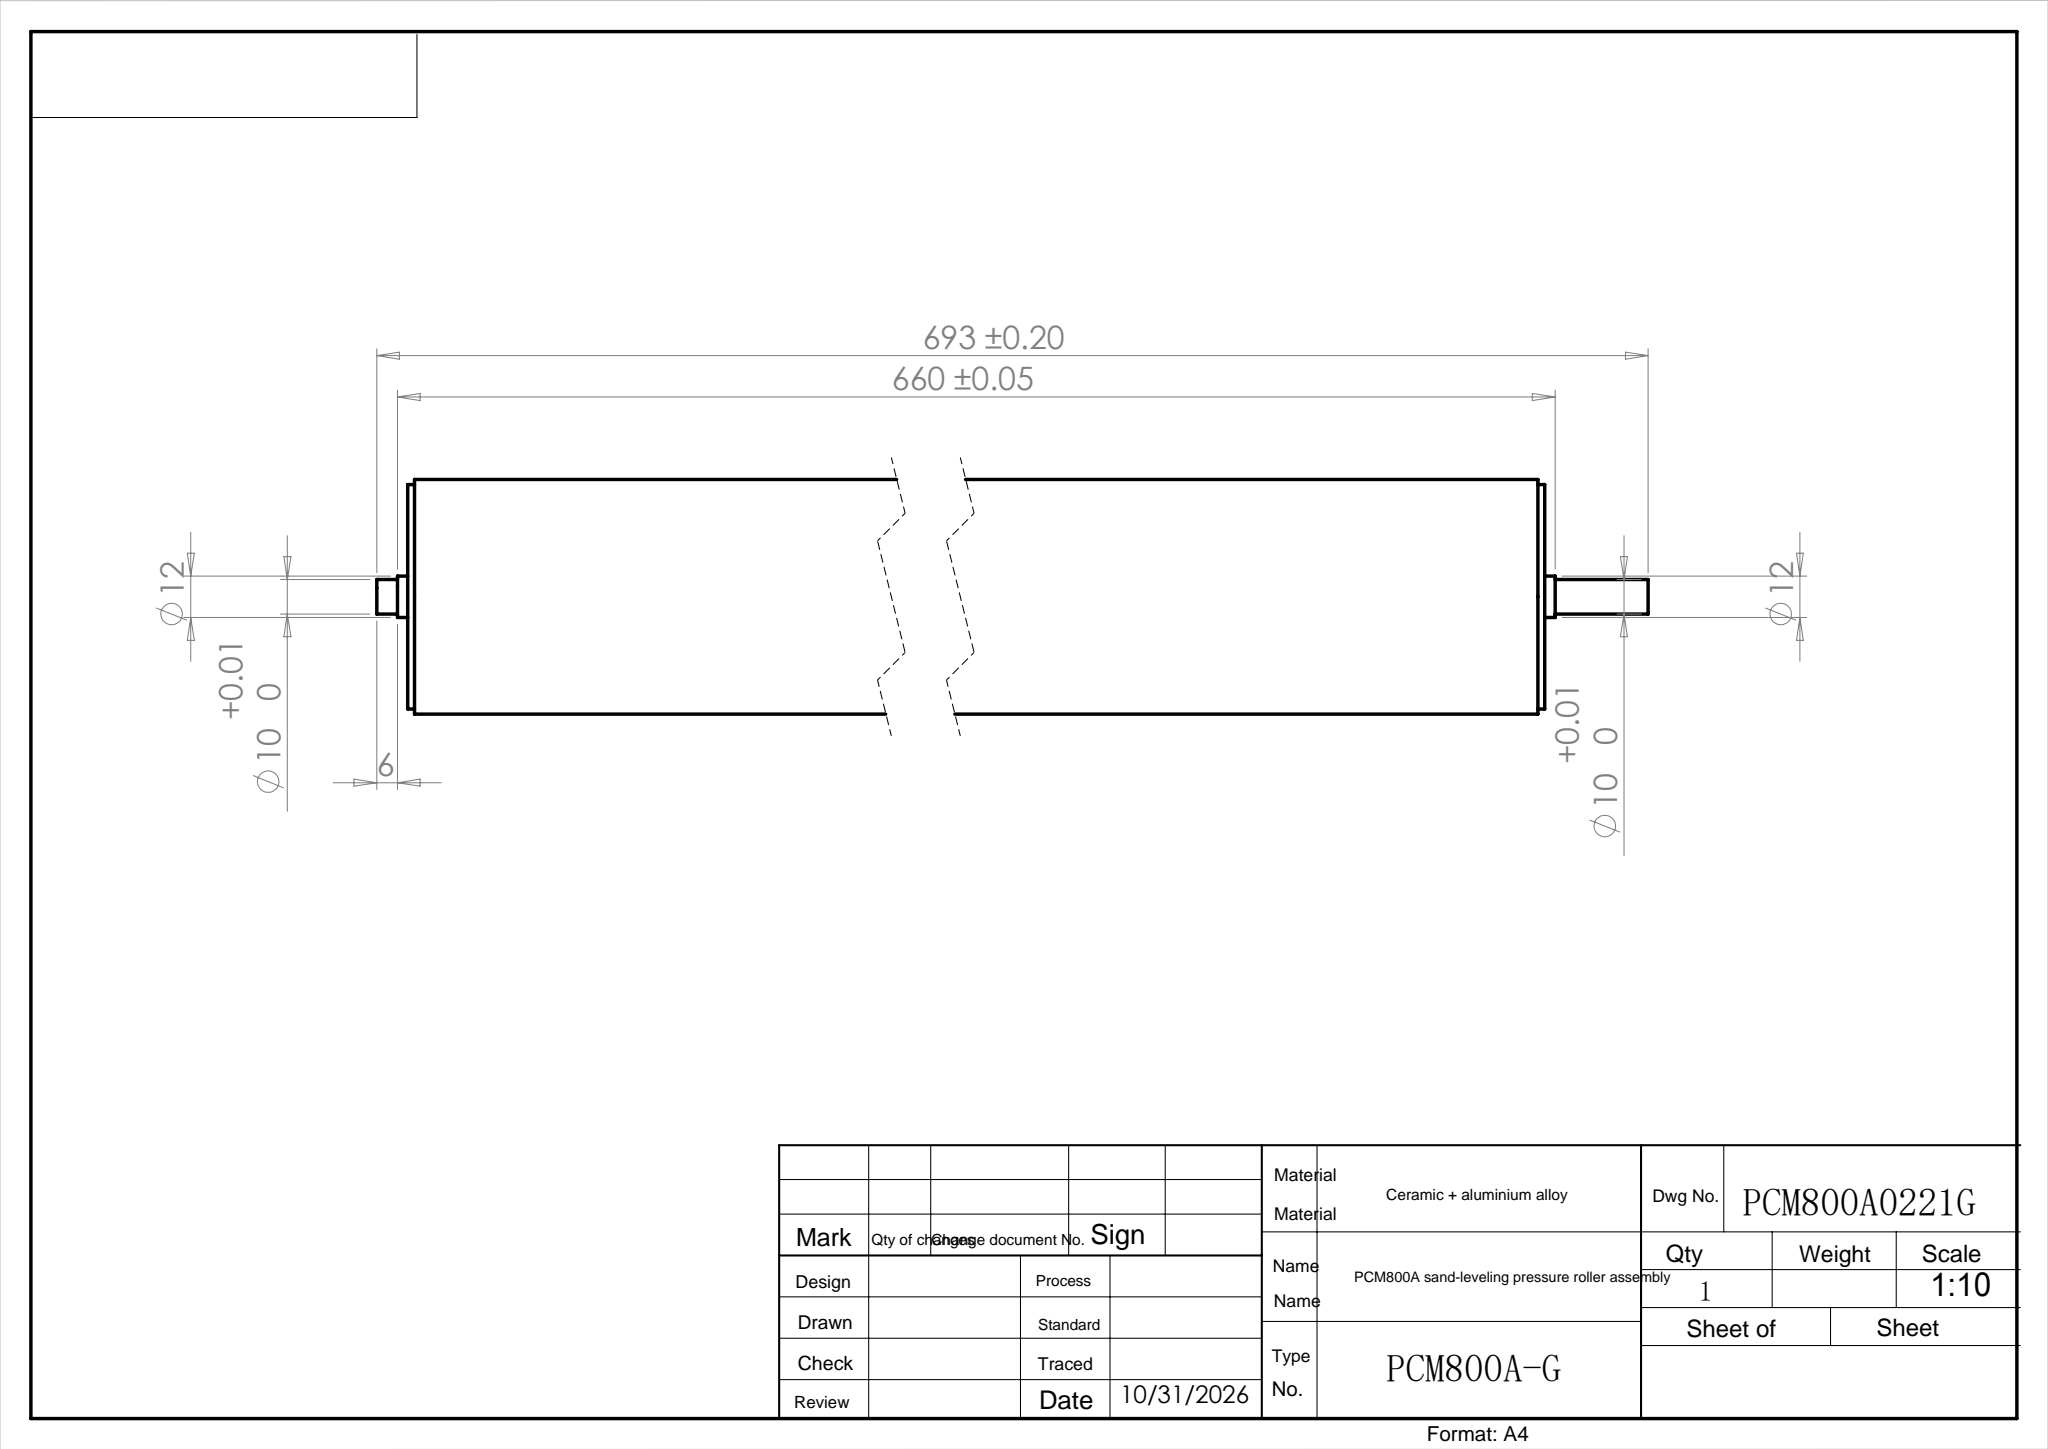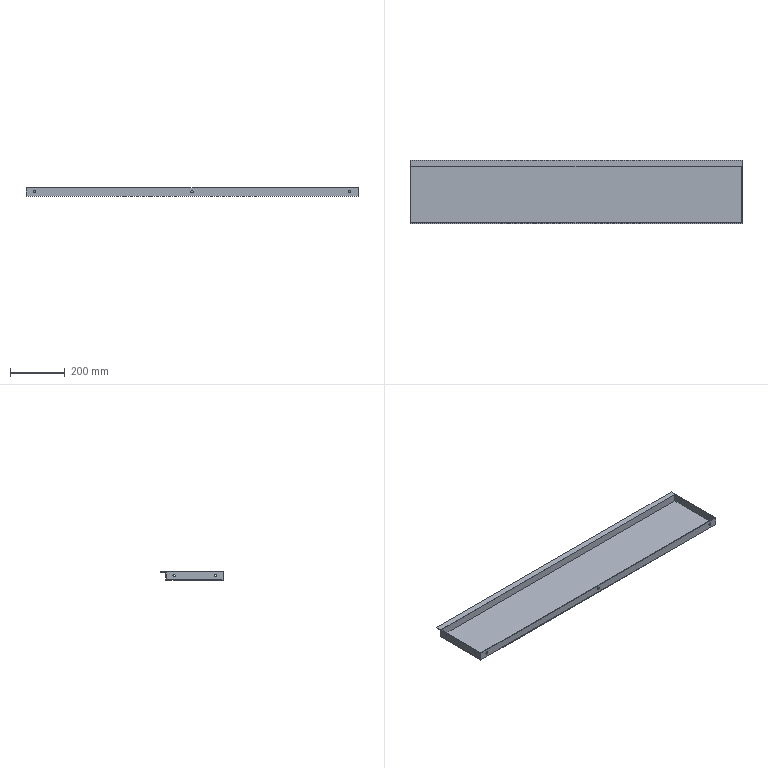Part | SolidWorks | features ICE 3, Extrusion 1, Shell 1 | 1 solid | 27 faces | box 1210 x 230 x 30 mm | volume 714301 mm3 | cylinder 14 | plane 13 | commonest cylinder face diameters 9 x14
STEP:
#1=CARTESIAN_POINT('',(2.,30.,11.5));
#2=VERTEX_POINT('',#1);
#3=CARTESIAN_POINT('',(2.,30.,20.5));
#4=VERTEX_POINT('',#3);
#5=CARTESIAN_POINT('',(2.,30.,16.));
#6=DIRECTION('',(-1.,0.,0.));
#7=DIRECTION('',(0.,0.,-1.));
#8=AXIS2_PLACEMENT_3D('',#5,#6,#7);
#9=CIRCLE('',#8,4.5);
#10=EDGE_CURVE('',#2,#4,#9,.T.);
#11=ORIENTED_EDGE('',*,*,#10,.F.);
#12=CARTESIAN_POINT('',(0.,30.,11.5));
#13=VERTEX_POINT('',#12);
#14=CARTESIAN_POINT('',(1517.,30.,11.5));
#15=DIRECTION('',(-1.,0.,0.));
#16=VECTOR('',#15,1000.);
#17=LINE('',#14,#16);
#18=EDGE_CURVE('',#2,#13,#17,.T.);
#19=ORIENTED_EDGE('',*,*,#18,.T.);
#20=CARTESIAN_POINT('',(0.,30.,20.5));
#21=VERTEX_POINT('',#20);
#22=CARTESIAN_POINT('',(0.,30.,16.));
#23=DIRECTION('',(-1.,0.,0.));
#24=DIRECTION('',(0.,0.,-1.));
#25=AXIS2_PLACEMENT_3D('',#22,#23,#24);
#26=CIRCLE('',#25,4.5);
#27=EDGE_CURVE('',#13,#21,#26,.T.);
#28=ORIENTED_EDGE('',*,*,#27,.T.);
#29=CARTESIAN_POINT('',(1517.,30.,20.5));
#30=DIRECTION('',(-1.,0.,0.));
#31=VECTOR('',#30,1000.);
#32=LINE('',#29,#31);
#33=EDGE_CURVE('',#4,#21,#32,.T.);
#34=ORIENTED_EDGE('',*,*,#33,.F.);
#35=EDGE_LOOP('',(#11,#19,#28,#34));
#36=FACE_OUTER_BOUND('',#35,.T.);
#37=CARTESIAN_POINT('',(1517.,30.,16.));
#38=DIRECTION('',(-1.,0.,0.));
#39=DIRECTION('',(0.,0.,1.));
#40=AXIS2_PLACEMENT_3D('',#37,#38,#39);
#41=CYLINDRICAL_SURFACE('',#40,4.5);
#42=ADVANCED_FACE('',(#36),#41,.F.);
#43=CARTESIAN_POINT('',(1210.,30.,20.5));
#44=VERTEX_POINT('',#43);
#45=CARTESIAN_POINT('',(1210.,30.,11.5));
#46=VERTEX_POINT('',#45);
#47=CARTESIAN_POINT('',(1210.,30.,16.));
#48=DIRECTION('',(1.,0.,0.));
#49=DIRECTION('',(0.,0.,1.));
#50=AXIS2_PLACEMENT_3D('',#47,#48,#49);
#51=CIRCLE('',#50,4.5);
#52=EDGE_CURVE('',#44,#46,#51,.T.);
#53=ORIENTED_EDGE('',*,*,#52,.T.);
#54=CARTESIAN_POINT('',(1208.,30.,11.5));
#55=VERTEX_POINT('',#54);
#56=CARTESIAN_POINT('',(1517.,30.,11.5));
#57=DIRECTION('',(-1.,0.,0.));
#58=VECTOR('',#57,1000.);
#59=LINE('',#56,#58);
#60=EDGE_CURVE('',#46,#55,#59,.T.);
#61=ORIENTED_EDGE('',*,*,#60,.T.);
#62=CARTESIAN_POINT('',(1208.,30.,20.5));
#63=VERTEX_POINT('',#62);
#64=CARTESIAN_POINT('',(1208.,30.,16.));
#65=DIRECTION('',(1.,0.,0.));
#66=DIRECTION('',(0.,0.,1.));
#67=AXIS2_PLACEMENT_3D('',#64,#65,#66);
#68=CIRCLE('',#67,4.5);
#69=EDGE_CURVE('',#63,#55,#68,.T.);
#70=ORIENTED_EDGE('',*,*,#69,.F.);
#71=CARTESIAN_POINT('',(1517.,30.,20.5));
#72=DIRECTION('',(-1.,0.,0.));
#73=VECTOR('',#72,1000.);
#74=LINE('',#71,#73);
#75=EDGE_CURVE('',#44,#63,#74,.T.);
#76=ORIENTED_EDGE('',*,*,#75,.F.);
#77=EDGE_LOOP('',(#53,#61,#70,#76));
#78=FACE_OUTER_BOUND('',#77,.T.);
#79=CARTESIAN_POINT('',(1517.,30.,16.));
#80=DIRECTION('',(-1.,0.,0.));
#81=DIRECTION('',(0.,0.,1.));
#82=AXIS2_PLACEMENT_3D('',#79,#80,#81);
#83=CYLINDRICAL_SURFACE('',#82,4.5);
#84=ADVANCED_FACE('',(#78),#83,.F.);
#85=CARTESIAN_POINT('',(2.,180.,11.5));
#86=VERTEX_POINT('',#85);
#87=CARTESIAN_POINT('',(2.,180.,20.5));
#88=VERTEX_POINT('',#87);
#89=CARTESIAN_POINT('',(2.,180.,16.));
#90=DIRECTION('',(-1.,0.,0.));
#91=DIRECTION('',(0.,0.,-1.));
#92=AXIS2_PLACEMENT_3D('',#89,#90,#91);
#93=CIRCLE('',#92,4.5);
#94=EDGE_CURVE('',#86,#88,#93,.T.);
#95=ORIENTED_EDGE('',*,*,#94,.F.);
#96=CARTESIAN_POINT('',(0.,180.,11.5));
#97=VERTEX_POINT('',#96);
#98=CARTESIAN_POINT('',(1517.,180.,11.5));
#99=DIRECTION('',(-1.,0.,0.));
#100=VECTOR('',#99,1000.);
#101=LINE('',#98,#100);
#102=EDGE_CURVE('',#86,#97,#101,.T.);
#103=ORIENTED_EDGE('',*,*,#102,.T.);
#104=CARTESIAN_POINT('',(0.,180.,20.5));
#105=VERTEX_POINT('',#104);
#106=CARTESIAN_POINT('',(0.,180.,16.));
#107=DIRECTION('',(-1.,0.,0.));
#108=DIRECTION('',(0.,0.,-1.));
#109=AXIS2_PLACEMENT_3D('',#106,#107,#108);
#110=CIRCLE('',#109,4.5);
#111=EDGE_CURVE('',#97,#105,#110,.T.);
#112=ORIENTED_EDGE('',*,*,#111,.T.);
#113=CARTESIAN_POINT('',(1517.,180.,20.5));
#114=DIRECTION('',(-1.,0.,0.));
#115=VECTOR('',#114,1000.);
#116=LINE('',#113,#115);
#117=EDGE_CURVE('',#88,#105,#116,.T.);
#118=ORIENTED_EDGE('',*,*,#117,.F.);
#119=EDGE_LOOP('',(#95,#103,#112,#118));
#120=FACE_OUTER_BOUND('',#119,.T.);
#121=CARTESIAN_POINT('',(1517.,180.,16.));
#122=DIRECTION('',(-1.,0.,0.));
#123=DIRECTION('',(0.,0.,1.));
#124=AXIS2_PLACEMENT_3D('',#121,#122,#123);
#125=CYLINDRICAL_SURFACE('',#124,4.5);
#126=ADVANCED_FACE('',(#120),#125,.F.);
#127=CARTESIAN_POINT('',(1210.,180.,20.5));
#128=VERTEX_POINT('',#127);
#129=CARTESIAN_POINT('',(1210.,180.,11.5));
#130=VERTEX_POINT('',#129);
#131=CARTESIAN_POINT('',(1210.,180.,16.));
#132=DIRECTION('',(1.,0.,0.));
#133=DIRECTION('',(0.,0.,1.));
#134=AXIS2_PLACEMENT_3D('',#131,#132,#133);
#135=CIRCLE('',#134,4.5);
#136=EDGE_CURVE('',#128,#130,#135,.T.);
#137=ORIENTED_EDGE('',*,*,#136,.T.);
#138=CARTESIAN_POINT('',(1208.,180.,11.5));
#139=VERTEX_POINT('',#138);
#140=CARTESIAN_POINT('',(1517.,180.,11.5));
#141=DIRECTION('',(-1.,0.,0.));
#142=VECTOR('',#141,1000.);
#143=LINE('',#140,#142);
#144=EDGE_CURVE('',#130,#139,#143,.T.);
#145=ORIENTED_EDGE('',*,*,#144,.T.);
#146=CARTESIAN_POINT('',(1208.,180.,20.5));
#147=VERTEX_POINT('',#146);
#148=CARTESIAN_POINT('',(1208.,180.,16.));
#149=DIRECTION('',(1.,0.,0.));
#150=DIRECTION('',(0.,0.,1.));
#151=AXIS2_PLACEMENT_3D('',#148,#149,#150);
#152=CIRCLE('',#151,4.5);
#153=EDGE_CURVE('',#147,#139,#152,.T.);
#154=ORIENTED_EDGE('',*,*,#153,.F.);
#155=CARTESIAN_POINT('',(1517.,180.,20.5));
#156=DIRECTION('',(-1.,0.,0.));
#157=VECTOR('',#156,1000.);
#158=LINE('',#155,#157);
#159=EDGE_CURVE('',#128,#147,#158,.T.);
#160=ORIENTED_EDGE('',*,*,#159,.F.);
#161=EDGE_LOOP('',(#137,#145,#154,#160));
#162=FACE_OUTER_BOUND('',#161,.T.);
#163=CARTESIAN_POINT('',(1517.,180.,16.));
#164=DIRECTION('',(-1.,0.,0.));
#165=DIRECTION('',(0.,0.,1.));
#166=AXIS2_PLACEMENT_3D('',#163,#164,#165);
#167=CYLINDRICAL_SURFACE('',#166,4.5);
#168=ADVANCED_FACE('',(#162),#167,.F.);
#169=CARTESIAN_POINT('',(605.,0.,11.5));
#170=VERTEX_POINT('',#169);
#171=CARTESIAN_POINT('',(605.,0.,20.5));
#172=VERTEX_POINT('',#171);
#173=CARTESIAN_POINT('',(605.,0.,16.));
#174=DIRECTION('',(0.,1.,0.));
#175=DIRECTION('',(0.,0.,1.));
#176=AXIS2_PLACEMENT_3D('',#173,#174,#175);
#177=CIRCLE('',#176,4.5);
#178=EDGE_CURVE('',#170,#172,#177,.T.);
#179=ORIENTED_EDGE('',*,*,#178,.F.);
#180=CARTESIAN_POINT('',(605.,2.,11.5));
#181=VERTEX_POINT('',#180);
#182=CARTESIAN_POINT('',(605.,-92.,11.5));
#183=DIRECTION('',(0.,1.,0.));
#184=VECTOR('',#183,1000.);
#185=LINE('',#182,#184);
#186=EDGE_CURVE('',#170,#181,#185,.T.);
#187=ORIENTED_EDGE('',*,*,#186,.T.);
#188=CARTESIAN_POINT('',(605.,2.,20.5));
#189=VERTEX_POINT('',#188);
#190=CARTESIAN_POINT('',(605.,2.,16.));
#191=DIRECTION('',(0.,1.,0.));
#192=DIRECTION('',(0.,0.,1.));
#193=AXIS2_PLACEMENT_3D('',#190,#191,#192);
#194=CIRCLE('',#193,4.5);
#195=EDGE_CURVE('',#181,#189,#194,.T.);
#196=ORIENTED_EDGE('',*,*,#195,.T.);
#197=CARTESIAN_POINT('',(605.,-92.,20.5));
#198=DIRECTION('',(0.,1.,0.));
#199=VECTOR('',#198,1000.);
#200=LINE('',#197,#199);
#201=EDGE_CURVE('',#172,#189,#200,.T.);
#202=ORIENTED_EDGE('',*,*,#201,.F.);
#203=EDGE_LOOP('',(#179,#187,#196,#202));
#204=FACE_OUTER_BOUND('',#203,.T.);
#205=CARTESIAN_POINT('',(605.,-92.,16.));
#206=DIRECTION('',(0.,1.,0.));
#207=DIRECTION('',(0.,0.,1.));
#208=AXIS2_PLACEMENT_3D('',#205,#206,#207);
#209=CYLINDRICAL_SURFACE('',#208,4.5);
#210=ADVANCED_FACE('',(#204),#209,.F.);
#211=CARTESIAN_POINT('',(30.,0.,11.5));
#212=VERTEX_POINT('',#211);
#213=CARTESIAN_POINT('',(30.,0.,20.5));
#214=VERTEX_POINT('',#213);
#215=CARTESIAN_POINT('',(30.,0.,16.));
#216=DIRECTION('',(0.,1.,0.));
#217=DIRECTION('',(0.,0.,1.));
#218=AXIS2_PLACEMENT_3D('',#215,#216,#217);
#219=CIRCLE('',#218,4.5);
#220=EDGE_CURVE('',#212,#214,#219,.T.);
#221=ORIENTED_EDGE('',*,*,#220,.F.);
#222=CARTESIAN_POINT('',(30.,2.,11.5));
#223=VERTEX_POINT('',#222);
#224=CARTESIAN_POINT('',(30.,-92.,11.5));
#225=DIRECTION('',(0.,1.,0.));
#226=VECTOR('',#225,1000.);
#227=LINE('',#224,#226);
#228=EDGE_CURVE('',#212,#223,#227,.T.);
#229=ORIENTED_EDGE('',*,*,#228,.T.);
#230=CARTESIAN_POINT('',(30.,2.,20.5));
#231=VERTEX_POINT('',#230);
#232=CARTESIAN_POINT('',(30.,2.,16.));
#233=DIRECTION('',(0.,1.,0.));
#234=DIRECTION('',(0.,0.,1.));
#235=AXIS2_PLACEMENT_3D('',#232,#233,#234);
#236=CIRCLE('',#235,4.5);
#237=EDGE_CURVE('',#223,#231,#236,.T.);
#238=ORIENTED_EDGE('',*,*,#237,.T.);
#239=CARTESIAN_POINT('',(30.,-92.,20.5));
#240=DIRECTION('',(0.,1.,0.));
#241=VECTOR('',#240,1000.);
#242=LINE('',#239,#241);
#243=EDGE_CURVE('',#214,#231,#242,.T.);
#244=ORIENTED_EDGE('',*,*,#243,.F.);
#245=EDGE_LOOP('',(#221,#229,#238,#244));
#246=FACE_OUTER_BOUND('',#245,.T.);
#247=CARTESIAN_POINT('',(30.,-92.,16.));
#248=DIRECTION('',(0.,1.,0.));
#249=DIRECTION('',(0.,0.,1.));
#250=AXIS2_PLACEMENT_3D('',#247,#248,#249);
#251=CYLINDRICAL_SURFACE('',#250,4.5);
#252=ADVANCED_FACE('',(#246),#251,.F.);
#253=CARTESIAN_POINT('',(1180.,0.,11.5));
#254=VERTEX_POINT('',#253);
#255=CARTESIAN_POINT('',(1180.,0.,20.5));
#256=VERTEX_POINT('',#255);
#257=CARTESIAN_POINT('',(1180.,0.,16.));
#258=DIRECTION('',(0.,1.,0.));
#259=DIRECTION('',(0.,0.,1.));
#260=AXIS2_PLACEMENT_3D('',#257,#258,#259);
#261=CIRCLE('',#260,4.5);
#262=EDGE_CURVE('',#254,#256,#261,.T.);
#263=ORIENTED_EDGE('',*,*,#262,.F.);
#264=CARTESIAN_POINT('',(1180.,2.,11.5));
#265=VERTEX_POINT('',#264);
#266=CARTESIAN_POINT('',(1180.,-92.,11.5));
#267=DIRECTION('',(0.,1.,0.));
#268=VECTOR('',#267,1000.);
#269=LINE('',#266,#268);
#270=EDGE_CURVE('',#254,#265,#269,.T.);
#271=ORIENTED_EDGE('',*,*,#270,.T.);
#272=CARTESIAN_POINT('',(1180.,2.,20.5));
#273=VERTEX_POINT('',#272);
#274=CARTESIAN_POINT('',(1180.,2.,16.));
#275=DIRECTION('',(0.,1.,0.));
#276=DIRECTION('',(0.,0.,1.));
#277=AXIS2_PLACEMENT_3D('',#274,#275,#276);
#278=CIRCLE('',#277,4.5);
#279=EDGE_CURVE('',#265,#273,#278,.T.);
#280=ORIENTED_EDGE('',*,*,#279,.T.);
#281=CARTESIAN_POINT('',(1180.,-92.,20.5));
#282=DIRECTION('',(0.,1.,0.));
#283=VECTOR('',#282,1000.);
#284=LINE('',#281,#283);
#285=EDGE_CURVE('',#256,#273,#284,.T.);
#286=ORIENTED_EDGE('',*,*,#285,.F.);
#287=EDGE_LOOP('',(#263,#271,#280,#286));
#288=FACE_OUTER_BOUND('',#287,.T.);
#289=CARTESIAN_POINT('',(1180.,-92.,16.));
#290=DIRECTION('',(0.,1.,0.));
#291=DIRECTION('',(0.,0.,1.));
#292=AXIS2_PLACEMENT_3D('',#289,#290,#291);
#293=CYLINDRICAL_SURFACE('',#292,4.5);
#294=ADVANCED_FACE('',(#288),#293,.F.);
#295=CARTESIAN_POINT('',(0.,180.,16.));
#296=DIRECTION('',(-1.,0.,0.));
#297=DIRECTION('',(0.,0.,-1.));
#298=AXIS2_PLACEMENT_3D('',#295,#296,#297);
#299=CIRCLE('',#298,4.5);
#300=EDGE_CURVE('',#105,#97,#299,.T.);
#301=ORIENTED_EDGE('',*,*,#300,.F.);
#302=ORIENTED_EDGE('',*,*,#111,.F.);
#303=EDGE_LOOP('',(#301,#302));
#304=FACE_BOUND('',#303,.T.);
#305=CARTESIAN_POINT('',(0.,210.,0.));
#306=VERTEX_POINT('',#305);
#307=CARTESIAN_POINT('',(0.,0.,0.));
#308=VERTEX_POINT('',#307);
#309=CARTESIAN_POINT('',(0.,0.,0.));
#310=DIRECTION('',(0.,-1.,0.));
#311=VECTOR('',#310,1000.);
#312=LINE('',#309,#311);
#313=EDGE_CURVE('',#306,#308,#312,.T.);
#314=ORIENTED_EDGE('',*,*,#313,.T.);
#315=CARTESIAN_POINT('',(0.,0.,30.));
#316=VERTEX_POINT('',#315);
#317=CARTESIAN_POINT('',(0.,0.,30.));
#318=DIRECTION('',(0.,0.,-1.));
#319=VECTOR('',#318,1000.);
#320=LINE('',#317,#319);
#321=EDGE_CURVE('',#316,#308,#320,.T.);
#322=ORIENTED_EDGE('',*,*,#321,.F.);
#323=CARTESIAN_POINT('',(0.,230.,30.));
#324=VERTEX_POINT('',#323);
#325=CARTESIAN_POINT('',(0.,0.,30.));
#326=DIRECTION('',(0.,-1.,0.));
#327=VECTOR('',#326,1000.);
#328=LINE('',#325,#327);
#329=EDGE_CURVE('',#324,#316,#328,.T.);
#330=ORIENTED_EDGE('',*,*,#329,.F.);
#331=CARTESIAN_POINT('',(0.,230.,28.));
#332=VERTEX_POINT('',#331);
#333=CARTESIAN_POINT('',(0.,230.,28.));
#334=DIRECTION('',(0.,0.,1.));
#335=VECTOR('',#334,1000.);
#336=LINE('',#333,#335);
#337=EDGE_CURVE('',#332,#324,#336,.T.);
#338=ORIENTED_EDGE('',*,*,#337,.F.);
#339=CARTESIAN_POINT('',(0.,210.,28.));
#340=VERTEX_POINT('',#339);
#341=CARTESIAN_POINT('',(0.,230.,28.));
#342=DIRECTION('',(0.,-1.,0.));
#343=VECTOR('',#342,1000.);
#344=LINE('',#341,#343);
#345=EDGE_CURVE('',#332,#340,#344,.T.);
#346=ORIENTED_EDGE('',*,*,#345,.T.);
#347=CARTESIAN_POINT('',(0.,210.,30.));
#348=DIRECTION('',(0.,0.,-1.));
#349=VECTOR('',#348,1000.);
#350=LINE('',#347,#349);
#351=EDGE_CURVE('',#340,#306,#350,.T.);
#352=ORIENTED_EDGE('',*,*,#351,.T.);
#353=EDGE_LOOP('',(#314,#322,#330,#338,#346,#352));
#354=FACE_OUTER_BOUND('',#353,.T.);
#355=CARTESIAN_POINT('',(0.,30.,16.));
#356=DIRECTION('',(-1.,0.,0.));
#357=DIRECTION('',(0.,0.,-1.));
#358=AXIS2_PLACEMENT_3D('',#355,#356,#357);
#359=CIRCLE('',#358,4.5);
#360=EDGE_CURVE('',#21,#13,#359,.T.);
#361=ORIENTED_EDGE('',*,*,#360,.F.);
#362=ORIENTED_EDGE('',*,*,#27,.F.);
#363=EDGE_LOOP('',(#361,#362));
#364=FACE_BOUND('',#363,.T.);
#365=CARTESIAN_POINT('',(0.,0.,30.));
#366=DIRECTION('',(1.,0.,0.));
#367=DIRECTION('',(0.,0.,-1.));
#368=AXIS2_PLACEMENT_3D('',#365,#366,#367);
#369=PLANE('',#368);
#370=ADVANCED_FACE('',(#304,#354,#364),#369,.F.);
#371=ORIENTED_EDGE('',*,*,#136,.F.);
#372=CARTESIAN_POINT('',(1210.,180.,16.));
#373=DIRECTION('',(1.,0.,0.));
#374=DIRECTION('',(0.,0.,1.));
#375=AXIS2_PLACEMENT_3D('',#372,#373,#374);
#376=CIRCLE('',#375,4.5);
#377=EDGE_CURVE('',#130,#128,#376,.T.);
#378=ORIENTED_EDGE('',*,*,#377,.F.);
#379=EDGE_LOOP('',(#371,#378));
#380=FACE_BOUND('',#379,.T.);
#381=CARTESIAN_POINT('',(1210.,0.,0.));
#382=VERTEX_POINT('',#381);
#383=CARTESIAN_POINT('',(1210.,210.,0.));
#384=VERTEX_POINT('',#383);
#385=CARTESIAN_POINT('',(1210.,0.,0.));
#386=DIRECTION('',(0.,1.,0.));
#387=VECTOR('',#386,1000.);
#388=LINE('',#385,#387);
#389=EDGE_CURVE('',#382,#384,#388,.T.);
#390=ORIENTED_EDGE('',*,*,#389,.T.);
#391=CARTESIAN_POINT('',(1210.,210.,28.));
#392=VERTEX_POINT('',#391);
#393=CARTESIAN_POINT('',(1210.,210.,30.));
#394=DIRECTION('',(0.,0.,-1.));
#395=VECTOR('',#394,1000.);
#396=LINE('',#393,#395);
#397=EDGE_CURVE('',#392,#384,#396,.T.);
#398=ORIENTED_EDGE('',*,*,#397,.F.);
#399=CARTESIAN_POINT('',(1210.,230.,28.));
#400=VERTEX_POINT('',#399);
#401=CARTESIAN_POINT('',(1210.,210.,28.));
#402=DIRECTION('',(0.,1.,0.));
#403=VECTOR('',#402,1000.);
#404=LINE('',#401,#403);
#405=EDGE_CURVE('',#392,#400,#404,.T.);
#406=ORIENTED_EDGE('',*,*,#405,.T.);
#407=CARTESIAN_POINT('',(1210.,230.,30.));
#408=VERTEX_POINT('',#407);
#409=CARTESIAN_POINT('',(1210.,230.,28.));
#410=DIRECTION('',(0.,0.,1.));
#411=VECTOR('',#410,1000.);
#412=LINE('',#409,#411);
#413=EDGE_CURVE('',#400,#408,#412,.T.);
#414=ORIENTED_EDGE('',*,*,#413,.T.);
#415=CARTESIAN_POINT('',(1210.,0.,30.));
#416=VERTEX_POINT('',#415);
#417=CARTESIAN_POINT('',(1210.,0.,30.));
#418=DIRECTION('',(0.,1.,0.));
#419=VECTOR('',#418,1000.);
#420=LINE('',#417,#419);
#421=EDGE_CURVE('',#416,#408,#420,.T.);
#422=ORIENTED_EDGE('',*,*,#421,.F.);
#423=CARTESIAN_POINT('',(1210.,0.,30.));
#424=DIRECTION('',(0.,0.,-1.));
#425=VECTOR('',#424,1000.);
#426=LINE('',#423,#425);
#427=EDGE_CURVE('',#416,#382,#426,.T.);
#428=ORIENTED_EDGE('',*,*,#427,.T.);
#429=EDGE_LOOP('',(#390,#398,#406,#414,#422,#428));
#430=FACE_OUTER_BOUND('',#429,.T.);
#431=ORIENTED_EDGE('',*,*,#52,.F.);
#432=CARTESIAN_POINT('',(1210.,30.,16.));
#433=DIRECTION('',(1.,0.,0.));
#434=DIRECTION('',(0.,0.,1.));
#435=AXIS2_PLACEMENT_3D('',#432,#433,#434);
#436=CIRCLE('',#435,4.5);
#437=EDGE_CURVE('',#46,#44,#436,.T.);
#438=ORIENTED_EDGE('',*,*,#437,.F.);
#439=EDGE_LOOP('',(#431,#438));
#440=FACE_BOUND('',#439,.T.);
#441=CARTESIAN_POINT('',(1210.,0.,30.));
#442=DIRECTION('',(-1.,0.,0.));
#443=DIRECTION('',(0.,0.,1.));
#444=AXIS2_PLACEMENT_3D('',#441,#442,#443);
#445=PLANE('',#444);
#446=ADVANCED_FACE('',(#380,#430,#440),#445,.F.);
#447=CARTESIAN_POINT('',(2.,180.,16.));
#448=DIRECTION('',(-1.,0.,0.));
#449=DIRECTION('',(0.,0.,-1.));
#450=AXIS2_PLACEMENT_3D('',#447,#448,#449);
#451=CIRCLE('',#450,4.5);
#452=EDGE_CURVE('',#88,#86,#451,.T.);
#453=ORIENTED_EDGE('',*,*,#452,.T.);
#454=ORIENTED_EDGE('',*,*,#94,.T.);
#455=EDGE_LOOP('',(#453,#454));
#456=FACE_BOUND('',#455,.T.);
#457=CARTESIAN_POINT('',(2.,208.,2.));
#458=VERTEX_POINT('',#457);
#459=CARTESIAN_POINT('',(2.,2.,2.));
#460=VERTEX_POINT('',#459);
#461=CARTESIAN_POINT('',(2.,210.,2.));
#462=DIRECTION('',(0.,-1.,0.));
#463=VECTOR('',#462,1000.);
#464=LINE('',#461,#463);
#465=EDGE_CURVE('',#458,#460,#464,.T.);
#466=ORIENTED_EDGE('',*,*,#465,.F.);
#467=CARTESIAN_POINT('',(2.,208.,30.));
#468=VERTEX_POINT('',#467);
#469=CARTESIAN_POINT('',(2.,208.,30.));
#470=DIRECTION('',(0.,0.,-1.));
#471=VECTOR('',#470,1000.);
#472=LINE('',#469,#471);
#473=EDGE_CURVE('',#468,#458,#472,.T.);
#474=ORIENTED_EDGE('',*,*,#473,.F.);
#475=CARTESIAN_POINT('',(2.,2.,30.));
#476=VERTEX_POINT('',#475);
#477=CARTESIAN_POINT('',(2.,210.,30.));
#478=DIRECTION('',(0.,-1.,0.));
#479=VECTOR('',#478,1000.);
#480=LINE('',#477,#479);
#481=EDGE_CURVE('',#468,#476,#480,.T.);
#482=ORIENTED_EDGE('',*,*,#481,.T.);
#483=CARTESIAN_POINT('',(2.,2.,30.));
#484=DIRECTION('',(0.,0.,-1.));
#485=VECTOR('',#484,1000.);
#486=LINE('',#483,#485);
#487=EDGE_CURVE('',#476,#460,#486,.T.);
#488=ORIENTED_EDGE('',*,*,#487,.T.);
#489=EDGE_LOOP('',(#466,#474,#482,#488));
#490=FACE_OUTER_BOUND('',#489,.T.);
#491=CARTESIAN_POINT('',(2.,30.,16.));
#492=DIRECTION('',(-1.,0.,0.));
#493=DIRECTION('',(0.,0.,-1.));
#494=AXIS2_PLACEMENT_3D('',#491,#492,#493);
#495=CIRCLE('',#494,4.5);
#496=EDGE_CURVE('',#4,#2,#495,.T.);
#497=ORIENTED_EDGE('',*,*,#496,.T.);
#498=ORIENTED_EDGE('',*,*,#10,.T.);
#499=EDGE_LOOP('',(#497,#498));
#500=FACE_BOUND('',#499,.T.);
#501=CARTESIAN_POINT('',(2.,0.,30.));
#502=DIRECTION('',(1.,0.,0.));
#503=DIRECTION('',(0.,0.,-1.));
#504=AXIS2_PLACEMENT_3D('',#501,#502,#503);
#505=PLANE('',#504);
#506=ADVANCED_FACE('',(#456,#490,#500),#505,.T.);
#507=ORIENTED_EDGE('',*,*,#153,.T.);
#508=CARTESIAN_POINT('',(1208.,180.,16.));
#509=DIRECTION('',(1.,0.,0.));
#510=DIRECTION('',(0.,0.,1.));
#511=AXIS2_PLACEMENT_3D('',#508,#509,#510);
#512=CIRCLE('',#511,4.5);
#513=EDGE_CURVE('',#139,#147,#512,.T.);
#514=ORIENTED_EDGE('',*,*,#513,.T.);
#515=EDGE_LOOP('',(#507,#514));
#516=FACE_BOUND('',#515,.T.);
#517=CARTESIAN_POINT('',(1208.,2.,2.));
#518=VERTEX_POINT('',#517);
#519=CARTESIAN_POINT('',(1208.,208.,2.));
#520=VERTEX_POINT('',#519);
#521=CARTESIAN_POINT('',(1208.,210.,2.));
#522=DIRECTION('',(0.,1.,0.));
#523=VECTOR('',#522,1000.);
#524=LINE('',#521,#523);
#525=EDGE_CURVE('',#518,#520,#524,.T.);
#526=ORIENTED_EDGE('',*,*,#525,.F.);
#527=CARTESIAN_POINT('',(1208.,2.,30.));
#528=VERTEX_POINT('',#527);
#529=CARTESIAN_POINT('',(1208.,2.,30.));
#530=DIRECTION('',(0.,0.,-1.));
#531=VECTOR('',#530,1000.);
#532=LINE('',#529,#531);
#533=EDGE_CURVE('',#528,#518,#532,.T.);
#534=ORIENTED_EDGE('',*,*,#533,.F.);
#535=CARTESIAN_POINT('',(1208.,208.,30.));
#536=VERTEX_POINT('',#535);
#537=CARTESIAN_POINT('',(1208.,210.,30.));
#538=DIRECTION('',(0.,1.,0.));
#539=VECTOR('',#538,1000.);
#540=LINE('',#537,#539);
#541=EDGE_CURVE('',#528,#536,#540,.T.);
#542=ORIENTED_EDGE('',*,*,#541,.T.);
#543=CARTESIAN_POINT('',(1208.,208.,30.));
#544=DIRECTION('',(0.,0.,-1.));
#545=VECTOR('',#544,1000.);
#546=LINE('',#543,#545);
#547=EDGE_CURVE('',#536,#520,#546,.T.);
#548=ORIENTED_EDGE('',*,*,#547,.T.);
#549=EDGE_LOOP('',(#526,#534,#542,#548));
#550=FACE_OUTER_BOUND('',#549,.T.);
#551=ORIENTED_EDGE('',*,*,#69,.T.);
#552=CARTESIAN_POINT('',(1208.,30.,16.));
#553=DIRECTION('',(1.,0.,0.));
#554=DIRECTION('',(0.,0.,1.));
#555=AXIS2_PLACEMENT_3D('',#552,#553,#554);
#556=CIRCLE('',#555,4.5);
#557=EDGE_CURVE('',#55,#63,#556,.T.);
#558=ORIENTED_EDGE('',*,*,#557,.T.);
#559=EDGE_LOOP('',(#551,#558));
#560=FACE_BOUND('',#559,.T.);
#561=CARTESIAN_POINT('',(1208.,0.,30.));
#562=DIRECTION('',(-1.,0.,0.));
#563=DIRECTION('',(0.,0.,1.));
#564=AXIS2_PLACEMENT_3D('',#561,#562,#563);
#565=PLANE('',#564);
#566=ADVANCED_FACE('',(#516,#550,#560),#565,.T.);
#567=ORIENTED_EDGE('',*,*,#329,.T.);
#568=CARTESIAN_POINT('',(0.,0.,30.));
#569=DIRECTION('',(1.,0.,0.));
#570=VECTOR('',#569,1000.);
#571=LINE('',#568,#570);
#572=EDGE_CURVE('',#316,#416,#571,.T.);
#573=ORIENTED_EDGE('',*,*,#572,.T.);
#574=ORIENTED_EDGE('',*,*,#421,.T.);
#575=CARTESIAN_POINT('',(0.,230.,30.));
#576=DIRECTION('',(-1.,0.,0.));
#577=VECTOR('',#576,1000.);
#578=LINE('',#575,#577);
#579=EDGE_CURVE('',#408,#324,#578,.T.);
#580=ORIENTED_EDGE('',*,*,#579,.T.);
#581=EDGE_LOOP('',(#567,#573,#574,#580));
#582=FACE_OUTER_BOUND('',#581,.T.);
#583=ORIENTED_EDGE('',*,*,#481,.F.);
#584=CARTESIAN_POINT('',(0.,208.,30.));
#585=DIRECTION('',(-1.,0.,0.));
#586=VECTOR('',#585,1000.);
#587=LINE('',#584,#586);
#588=EDGE_CURVE('',#536,#468,#587,.T.);
#589=ORIENTED_EDGE('',*,*,#588,.F.);
#590=ORIENTED_EDGE('',*,*,#541,.F.);
#591=CARTESIAN_POINT('',(0.,2.,30.));
#592=DIRECTION('',(1.,0.,0.));
#593=VECTOR('',#592,1000.);
#594=LINE('',#591,#593);
#595=EDGE_CURVE('',#476,#528,#594,.T.);
#596=ORIENTED_EDGE('',*,*,#595,.F.);
#597=EDGE_LOOP('',(#583,#589,#590,#596));
#598=FACE_BOUND('',#597,.T.);
#599=CARTESIAN_POINT('',(0.,210.,30.));
#600=DIRECTION('',(0.,0.,-1.));
#601=DIRECTION('',(-1.,0.,0.));
#602=AXIS2_PLACEMENT_3D('',#599,#600,#601);
#603=PLANE('',#602);
#604=ADVANCED_FACE('',(#582,#598),#603,.F.);
#605=CARTESIAN_POINT('',(605.,0.,16.));
#606=DIRECTION('',(0.,1.,0.));
#607=DIRECTION('',(0.,0.,1.));
#608=AXIS2_PLACEMENT_3D('',#605,#606,#607);
#609=CIRCLE('',#608,4.5);
#610=EDGE_CURVE('',#172,#170,#609,.T.);
#611=ORIENTED_EDGE('',*,*,#610,.T.);
#612=ORIENTED_EDGE('',*,*,#178,.T.);
#613=EDGE_LOOP('',(#611,#612));
#614=FACE_BOUND('',#613,.T.);
#615=CARTESIAN_POINT('',(30.,0.,16.));
#616=DIRECTION('',(0.,1.,0.));
#617=DIRECTION('',(0.,0.,1.));
#618=AXIS2_PLACEMENT_3D('',#615,#616,#617);
#619=CIRCLE('',#618,4.5);
#620=EDGE_CURVE('',#214,#212,#619,.T.);
#621=ORIENTED_EDGE('',*,*,#620,.T.);
#622=ORIENTED_EDGE('',*,*,#220,.T.);
#623=EDGE_LOOP('',(#621,#622));
#624=FACE_BOUND('',#623,.T.);
#625=CARTESIAN_POINT('',(1180.,0.,16.));
#626=DIRECTION('',(0.,1.,0.));
#627=DIRECTION('',(0.,0.,1.));
#628=AXIS2_PLACEMENT_3D('',#625,#626,#627);
#629=CIRCLE('',#628,4.5);
#630=EDGE_CURVE('',#256,#254,#629,.T.);
#631=ORIENTED_EDGE('',*,*,#630,.T.);
#632=ORIENTED_EDGE('',*,*,#262,.T.);
#633=EDGE_LOOP('',(#631,#632));
#634=FACE_BOUND('',#633,.T.);
#635=CARTESIAN_POINT('',(0.,0.,0.));
#636=DIRECTION('',(1.,0.,0.));
#637=VECTOR('',#636,1000.);
#638=LINE('',#635,#637);
#639=EDGE_CURVE('',#308,#382,#638,.T.);
#640=ORIENTED_EDGE('',*,*,#639,.T.);
#641=ORIENTED_EDGE('',*,*,#427,.F.);
#642=ORIENTED_EDGE('',*,*,#572,.F.);
#643=ORIENTED_EDGE('',*,*,#321,.T.);
#644=EDGE_LOOP('',(#640,#641,#642,#643));
#645=FACE_OUTER_BOUND('',#644,.T.);
#646=CARTESIAN_POINT('',(0.,0.,30.));
#647=DIRECTION('',(0.,1.,0.));
#648=DIRECTION('',(0.,0.,1.));
#649=AXIS2_PLACEMENT_3D('',#646,#647,#648);
#650=PLANE('',#649);
#651=ADVANCED_FACE('',(#614,#624,#634,#645),#650,.F.);
#652=ORIENTED_EDGE('',*,*,#351,.F.);
#653=CARTESIAN_POINT('',(0.,210.,28.));
#654=DIRECTION('',(1.,0.,0.));
#655=VECTOR('',#654,1000.);
#656=LINE('',#653,#655);
#657=EDGE_CURVE('',#340,#392,#656,.T.);
#658=ORIENTED_EDGE('',*,*,#657,.T.);
#659=ORIENTED_EDGE('',*,*,#397,.T.);
#660=CARTESIAN_POINT('',(0.,210.,0.));
#661=DIRECTION('',(-1.,0.,0.));
#662=VECTOR('',#661,1000.);
#663=LINE('',#660,#662);
#664=EDGE_CURVE('',#384,#306,#663,.T.);
#665=ORIENTED_EDGE('',*,*,#664,.T.);
#666=EDGE_LOOP('',(#652,#658,#659,#665));
#667=FACE_OUTER_BOUND('',#666,.T.);
#668=CARTESIAN_POINT('',(0.,210.,30.));
#669=DIRECTION('',(0.,-1.,0.));
#670=DIRECTION('',(0.,0.,-1.));
#671=AXIS2_PLACEMENT_3D('',#668,#669,#670);
#672=PLANE('',#671);
#673=ADVANCED_FACE('',(#667),#672,.F.);
#674=ORIENTED_EDGE('',*,*,#313,.F.);
#675=ORIENTED_EDGE('',*,*,#664,.F.);
#676=ORIENTED_EDGE('',*,*,#389,.F.);
#677=ORIENTED_EDGE('',*,*,#639,.F.);
#678=EDGE_LOOP('',(#674,#675,#676,#677));
#679=FACE_OUTER_BOUND('',#678,.T.);
#680=CARTESIAN_POINT('',(0.,210.,0.));
#681=DIRECTION('',(0.,0.,-1.));
#682=DIRECTION('',(-1.,0.,0.));
#683=AXIS2_PLACEMENT_3D('',#680,#681,#682);
#684=PLANE('',#683);
#685=ADVANCED_FACE('',(#679),#684,.T.);
#686=CARTESIAN_POINT('',(605.,2.,16.));
#687=DIRECTION('',(0.,1.,0.));
#688=DIRECTION('',(0.,0.,1.));
#689=AXIS2_PLACEMENT_3D('',#686,#687,#688);
#690=CIRCLE('',#689,4.5);
#691=EDGE_CURVE('',#189,#181,#690,.T.);
#692=ORIENTED_EDGE('',*,*,#691,.F.);
#693=ORIENTED_EDGE('',*,*,#195,.F.);
#694=EDGE_LOOP('',(#692,#693));
#695=FACE_BOUND('',#694,.T.);
#696=CARTESIAN_POINT('',(30.,2.,16.));
#697=DIRECTION('',(0.,1.,0.));
#698=DIRECTION('',(0.,0.,1.));
#699=AXIS2_PLACEMENT_3D('',#696,#697,#698);
#700=CIRCLE('',#699,4.5);
#701=EDGE_CURVE('',#231,#223,#700,.T.);
#702=ORIENTED_EDGE('',*,*,#701,.F.);
#703=ORIENTED_EDGE('',*,*,#237,.F.);
#704=EDGE_LOOP('',(#702,#703));
#705=FACE_BOUND('',#704,.T.);
#706=CARTESIAN_POINT('',(1180.,2.,16.));
#707=DIRECTION('',(0.,1.,0.));
#708=DIRECTION('',(0.,0.,1.));
#709=AXIS2_PLACEMENT_3D('',#706,#707,#708);
#710=CIRCLE('',#709,4.5);
#711=EDGE_CURVE('',#273,#265,#710,.T.);
#712=ORIENTED_EDGE('',*,*,#711,.F.);
#713=ORIENTED_EDGE('',*,*,#279,.F.);
#714=EDGE_LOOP('',(#712,#713));
#715=FACE_BOUND('',#714,.T.);
#716=CARTESIAN_POINT('',(0.,2.,2.));
#717=DIRECTION('',(1.,0.,0.));
#718=VECTOR('',#717,1000.);
#719=LINE('',#716,#718);
#720=EDGE_CURVE('',#460,#518,#719,.T.);
#721=ORIENTED_EDGE('',*,*,#720,.F.);
#722=ORIENTED_EDGE('',*,*,#487,.F.);
#723=ORIENTED_EDGE('',*,*,#595,.T.);
#724=ORIENTED_EDGE('',*,*,#533,.T.);
#725=EDGE_LOOP('',(#721,#722,#723,#724));
#726=FACE_OUTER_BOUND('',#725,.T.);
#727=CARTESIAN_POINT('',(0.,2.,30.));
#728=DIRECTION('',(0.,1.,0.));
#729=DIRECTION('',(0.,0.,1.));
#730=AXIS2_PLACEMENT_3D('',#727,#728,#729);
#731=PLANE('',#730);
#732=ADVANCED_FACE('',(#695,#705,#715,#726),#731,.T.);
#733=CARTESIAN_POINT('',(0.,208.,2.));
#734=DIRECTION('',(-1.,0.,0.));
#735=VECTOR('',#734,1000.);
#736=LINE('',#733,#735);
#737=EDGE_CURVE('',#520,#458,#736,.T.);
#738=ORIENTED_EDGE('',*,*,#737,.F.);
#739=ORIENTED_EDGE('',*,*,#547,.F.);
#740=ORIENTED_EDGE('',*,*,#588,.T.);
#741=ORIENTED_EDGE('',*,*,#473,.T.);
#742=EDGE_LOOP('',(#738,#739,#740,#741));
#743=FACE_OUTER_BOUND('',#742,.T.);
#744=CARTESIAN_POINT('',(0.,208.,30.));
#745=DIRECTION('',(0.,-1.,0.));
#746=DIRECTION('',(0.,0.,-1.));
#747=AXIS2_PLACEMENT_3D('',#744,#745,#746);
#748=PLANE('',#747);
#749=ADVANCED_FACE('',(#743),#748,.T.);
#750=ORIENTED_EDGE('',*,*,#465,.T.);
#751=ORIENTED_EDGE('',*,*,#720,.T.);
#752=ORIENTED_EDGE('',*,*,#525,.T.);
#753=ORIENTED_EDGE('',*,*,#737,.T.);
#754=EDGE_LOOP('',(#750,#751,#752,#753));
#755=FACE_OUTER_BOUND('',#754,.T.);
#756=CARTESIAN_POINT('',(0.,210.,2.));
#757=DIRECTION('',(0.,0.,-1.));
#758=DIRECTION('',(-1.,0.,0.));
#759=AXIS2_PLACEMENT_3D('',#756,#757,#758);
#760=PLANE('',#759);
#761=ADVANCED_FACE('',(#755),#760,.F.);
#762=ORIENTED_EDGE('',*,*,#579,.F.);
#763=ORIENTED_EDGE('',*,*,#413,.F.);
#764=CARTESIAN_POINT('',(0.,230.,28.));
#765=DIRECTION('',(-1.,0.,0.));
#766=VECTOR('',#765,1000.);
#767=LINE('',#764,#766);
#768=EDGE_CURVE('',#400,#332,#767,.T.);
#769=ORIENTED_EDGE('',*,*,#768,.T.);
#770=ORIENTED_EDGE('',*,*,#337,.T.);
#771=EDGE_LOOP('',(#762,#763,#769,#770));
#772=FACE_OUTER_BOUND('',#771,.T.);
#773=CARTESIAN_POINT('',(0.,230.,28.));
#774=DIRECTION('',(0.,1.,0.));
#775=DIRECTION('',(-1.,0.,0.));
#776=AXIS2_PLACEMENT_3D('',#773,#774,#775);
#777=PLANE('',#776);
#778=ADVANCED_FACE('',(#772),#777,.T.);
#779=ORIENTED_EDGE('',*,*,#345,.F.);
#780=ORIENTED_EDGE('',*,*,#768,.F.);
#781=ORIENTED_EDGE('',*,*,#405,.F.);
#782=ORIENTED_EDGE('',*,*,#657,.F.);
#783=EDGE_LOOP('',(#779,#780,#781,#782));
#784=FACE_OUTER_BOUND('',#783,.T.);
#785=CARTESIAN_POINT('',(0.,210.,28.));
#786=DIRECTION('',(0.,0.,1.));
#787=DIRECTION('',(1.,0.,0.));
#788=AXIS2_PLACEMENT_3D('',#785,#786,#787);
#789=PLANE('',#788);
#790=ADVANCED_FACE('',(#784),#789,.F.);
#791=ORIENTED_EDGE('',*,*,#270,.F.);
#792=ORIENTED_EDGE('',*,*,#630,.F.);
#793=ORIENTED_EDGE('',*,*,#285,.T.);
#794=ORIENTED_EDGE('',*,*,#711,.T.);
#795=EDGE_LOOP('',(#791,#792,#793,#794));
#796=FACE_OUTER_BOUND('',#795,.T.);
#797=CARTESIAN_POINT('',(1180.,-92.,16.));
#798=DIRECTION('',(0.,1.,0.));
#799=DIRECTION('',(0.,0.,1.));
#800=AXIS2_PLACEMENT_3D('',#797,#798,#799);
#801=CYLINDRICAL_SURFACE('',#800,4.5);
#802=ADVANCED_FACE('',(#796),#801,.F.);
#803=ORIENTED_EDGE('',*,*,#228,.F.);
#804=ORIENTED_EDGE('',*,*,#620,.F.);
#805=ORIENTED_EDGE('',*,*,#243,.T.);
#806=ORIENTED_EDGE('',*,*,#701,.T.);
#807=EDGE_LOOP('',(#803,#804,#805,#806));
#808=FACE_OUTER_BOUND('',#807,.T.);
#809=CARTESIAN_POINT('',(30.,-92.,16.));
#810=DIRECTION('',(0.,1.,0.));
#811=DIRECTION('',(0.,0.,1.));
#812=AXIS2_PLACEMENT_3D('',#809,#810,#811);
#813=CYLINDRICAL_SURFACE('',#812,4.5);
#814=ADVANCED_FACE('',(#808),#813,.F.);
#815=ORIENTED_EDGE('',*,*,#186,.F.);
#816=ORIENTED_EDGE('',*,*,#610,.F.);
#817=ORIENTED_EDGE('',*,*,#201,.T.);
#818=ORIENTED_EDGE('',*,*,#691,.T.);
#819=EDGE_LOOP('',(#815,#816,#817,#818));
#820=FACE_OUTER_BOUND('',#819,.T.);
#821=CARTESIAN_POINT('',(605.,-92.,16.));
#822=DIRECTION('',(0.,1.,0.));
#823=DIRECTION('',(0.,0.,1.));
#824=AXIS2_PLACEMENT_3D('',#821,#822,#823);
#825=CYLINDRICAL_SURFACE('',#824,4.5);
#826=ADVANCED_FACE('',(#820),#825,.F.);
#827=ORIENTED_EDGE('',*,*,#144,.F.);
#828=ORIENTED_EDGE('',*,*,#377,.T.);
#829=ORIENTED_EDGE('',*,*,#159,.T.);
#830=ORIENTED_EDGE('',*,*,#513,.F.);
#831=EDGE_LOOP('',(#827,#828,#829,#830));
#832=FACE_OUTER_BOUND('',#831,.T.);
#833=CARTESIAN_POINT('',(1517.,180.,16.));
#834=DIRECTION('',(-1.,0.,0.));
#835=DIRECTION('',(0.,0.,1.));
#836=AXIS2_PLACEMENT_3D('',#833,#834,#835);
#837=CYLINDRICAL_SURFACE('',#836,4.5);
#838=ADVANCED_FACE('',(#832),#837,.F.);
#839=ORIENTED_EDGE('',*,*,#102,.F.);
#840=ORIENTED_EDGE('',*,*,#452,.F.);
#841=ORIENTED_EDGE('',*,*,#117,.T.);
#842=ORIENTED_EDGE('',*,*,#300,.T.);
#843=EDGE_LOOP('',(#839,#840,#841,#842));
#844=FACE_OUTER_BOUND('',#843,.T.);
#845=CARTESIAN_POINT('',(1517.,180.,16.));
#846=DIRECTION('',(-1.,0.,0.));
#847=DIRECTION('',(0.,0.,1.));
#848=AXIS2_PLACEMENT_3D('',#845,#846,#847);
#849=CYLINDRICAL_SURFACE('',#848,4.5);
#850=ADVANCED_FACE('',(#844),#849,.F.);
#851=ORIENTED_EDGE('',*,*,#60,.F.);
#852=ORIENTED_EDGE('',*,*,#437,.T.);
#853=ORIENTED_EDGE('',*,*,#75,.T.);
#854=ORIENTED_EDGE('',*,*,#557,.F.);
#855=EDGE_LOOP('',(#851,#852,#853,#854));
#856=FACE_OUTER_BOUND('',#855,.T.);
#857=CARTESIAN_POINT('',(1517.,30.,16.));
#858=DIRECTION('',(-1.,0.,0.));
#859=DIRECTION('',(0.,0.,1.));
#860=AXIS2_PLACEMENT_3D('',#857,#858,#859);
#861=CYLINDRICAL_SURFACE('',#860,4.5);
#862=ADVANCED_FACE('',(#856),#861,.F.);
#863=ORIENTED_EDGE('',*,*,#18,.F.);
#864=ORIENTED_EDGE('',*,*,#496,.F.);
#865=ORIENTED_EDGE('',*,*,#33,.T.);
#866=ORIENTED_EDGE('',*,*,#360,.T.);
#867=EDGE_LOOP('',(#863,#864,#865,#866));
#868=FACE_OUTER_BOUND('',#867,.T.);
#869=CARTESIAN_POINT('',(1517.,30.,16.));
#870=DIRECTION('',(-1.,0.,0.));
#871=DIRECTION('',(0.,0.,1.));
#872=AXIS2_PLACEMENT_3D('',#869,#870,#871);
#873=CYLINDRICAL_SURFACE('',#872,4.5);
#874=ADVANCED_FACE('',(#868),#873,.F.);
#875=CLOSED_SHELL('',(#42,#84,#126,#168,#210,#252,#294,#370,#446,#506,#566,#604,#651,#673,#685,#732,#749,#761,#778,#790,#802,#814,#826,#838,#850,#862,#874));
#876=MANIFOLD_SOLID_BREP('',#875);
#877=CARTESIAN_POINT('',(0.,0.,0.));
#878=DIRECTION('',(0.,0.,1.));
#879=DIRECTION('',(1.,0.,0.));
#880=AXIS2_PLACEMENT_3D('',#877,#878,#879);
#881=(LENGTH_UNIT()NAMED_UNIT(*)SI_UNIT(.MILLI.,.METRE.));
#882=UNCERTAINTY_MEASURE_WITH_UNIT(LENGTH_MEASURE(0.00001),#881,'','');
#883=(NAMED_UNIT(*)PLANE_ANGLE_UNIT()SI_UNIT($,.RADIAN.));
#884=(NAMED_UNIT(*)SI_UNIT($,.STERADIAN.)SOLID_ANGLE_UNIT());
#885=(GEOMETRIC_REPRESENTATION_CONTEXT(3)GLOBAL_UNCERTAINTY_ASSIGNED_CONTEXT((#882))GLOBAL_UNIT_ASSIGNED_CONTEXT((#881,#883,#884))REPRESENTATION_CONTEXT('',''));
#886=ADVANCED_BREP_SHAPE_REPRESENTATION('',(#876,#880),#885);